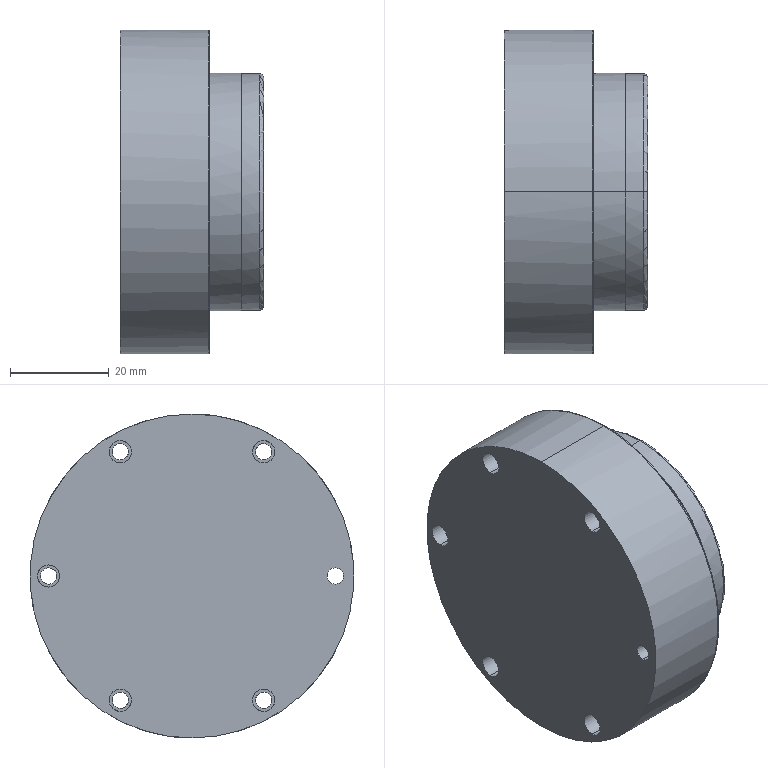Part | STEP file | 1 solid | 41 faces | box 29 x 65.5 x 65.5 mm | volume 78909 mm3 | cylinder 30 | plane 9 | torus 2 | commonest cylinder face diameters 3.3 x12 4.5 x10 65.5 x4 47.8 x2 48 x2